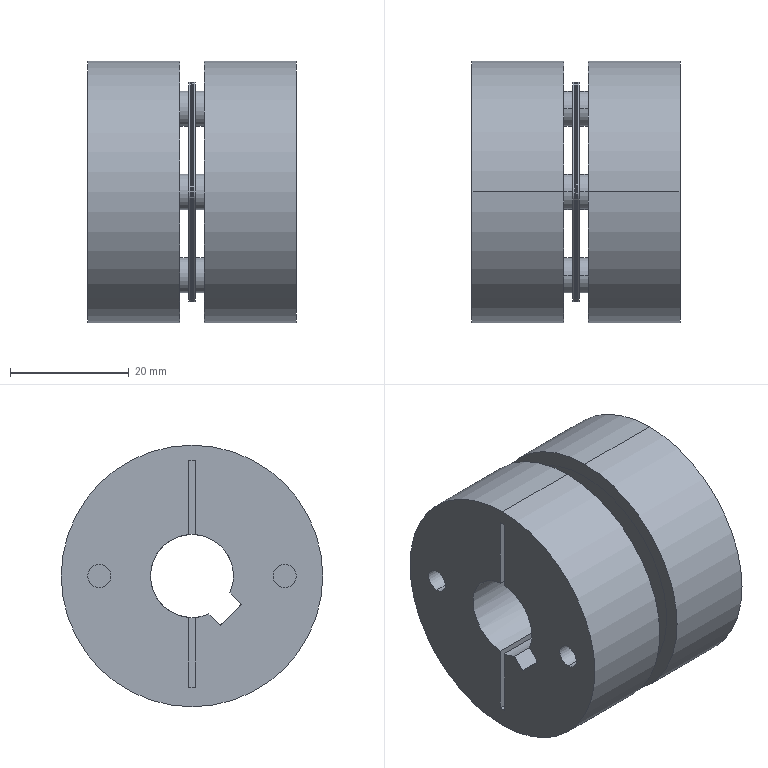Part | SolidWorks | features BaseBody 10 | 10 solids | 267 faces | box 35 x 44 x 44 mm | volume 38152 mm3 | cylinder 140 | plane 119 | spline 8 | commonest cylinder face diameters 5.938 x58 3.9 x33 19 x14 39 x11 4 x10 6.2 x6